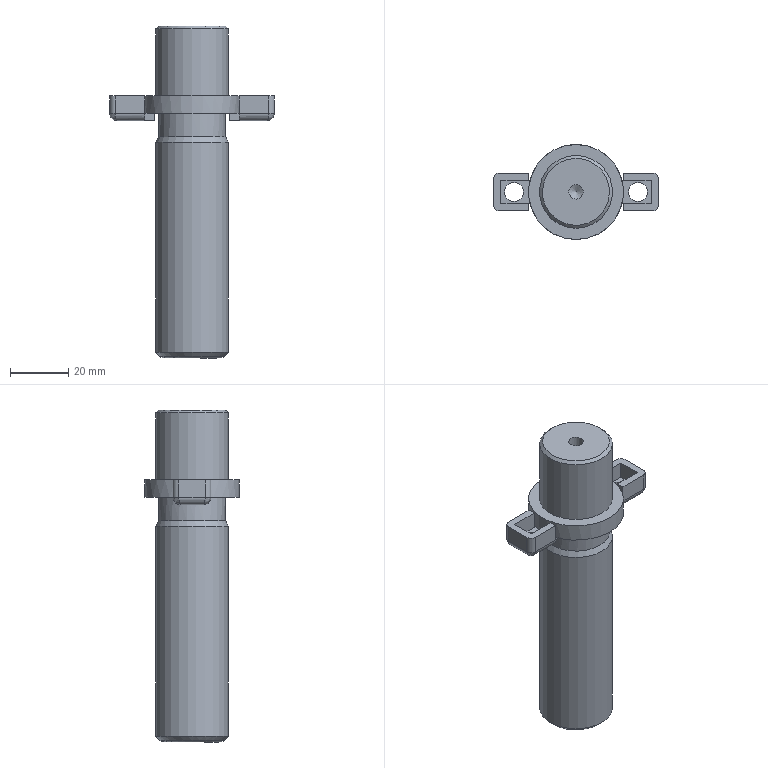Part | STEP file | gslz 2016.10.28-6_id434_x_t | 1 solid | 58 faces | box 56.6 x 32.6 x 114 mm | volume 58332 mm3 | plane 32 | cylinder 17 | cone 4 | spline 4 | torus 1 | commonest cylinder face diameters 5 x7 4 x4 6.5 x2 25 x2 23 x1 32.6 x1